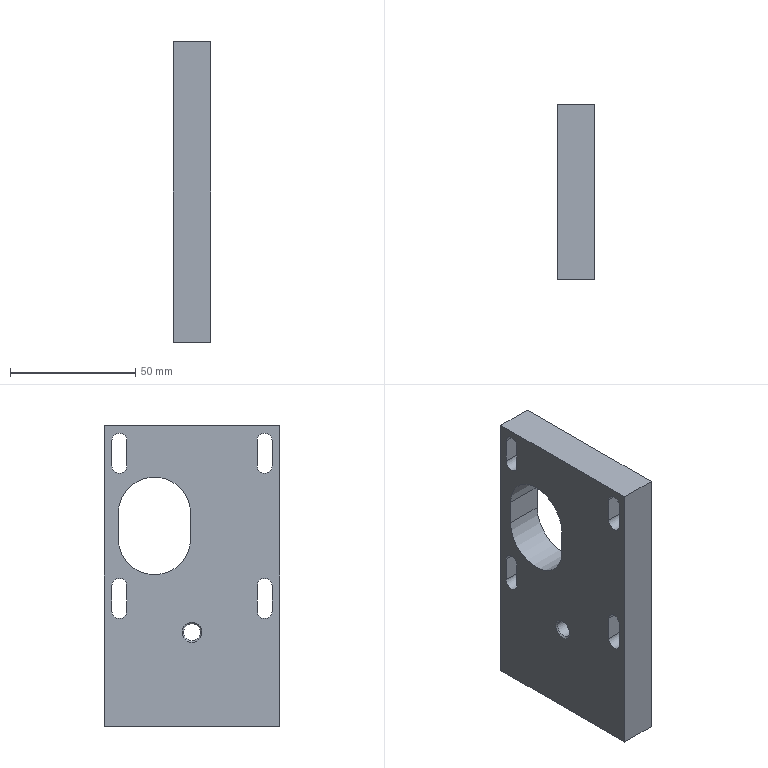Part | STEP file | YBQDJ-SSJ-9 | 1 solid | 35 faces | box 15 x 70 x 120 mm | volume 105388 mm3 | plane 16 | cylinder 13 | cone 6 | commonest cylinder face diameters 6 x8 5 x2 29 x2 6.8 x1